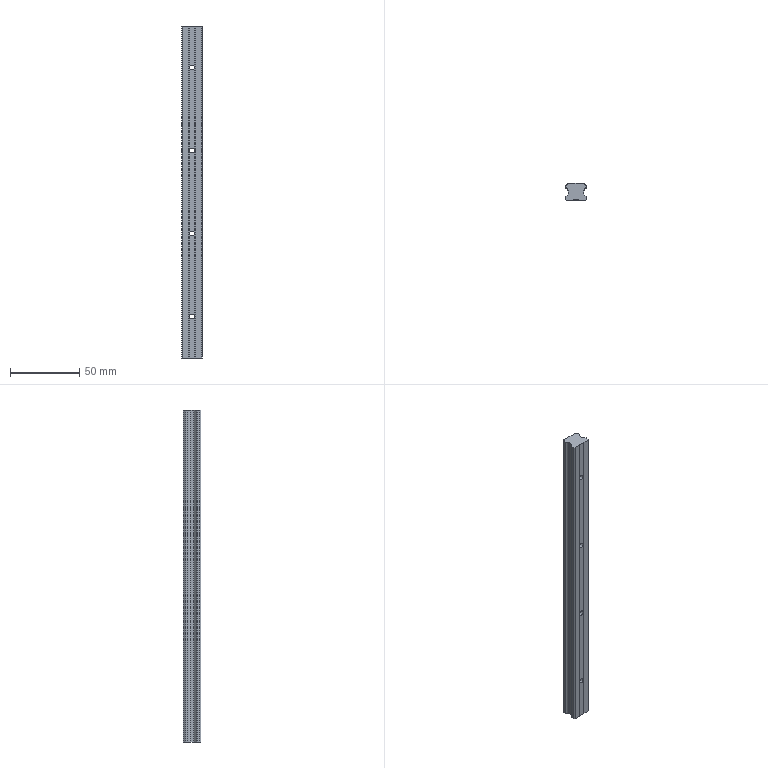Part | STEP file | EGH15CA2R600Z0C | 1 solid | 182 faces | box 15 x 12.5 x 240 mm | volume 38381 mm3 | plane 92 | spline 57 | cylinder 33 | commonest cylinder face diameters 0.6 x10 3.5 x8 6 x8 3 x5 1 x2